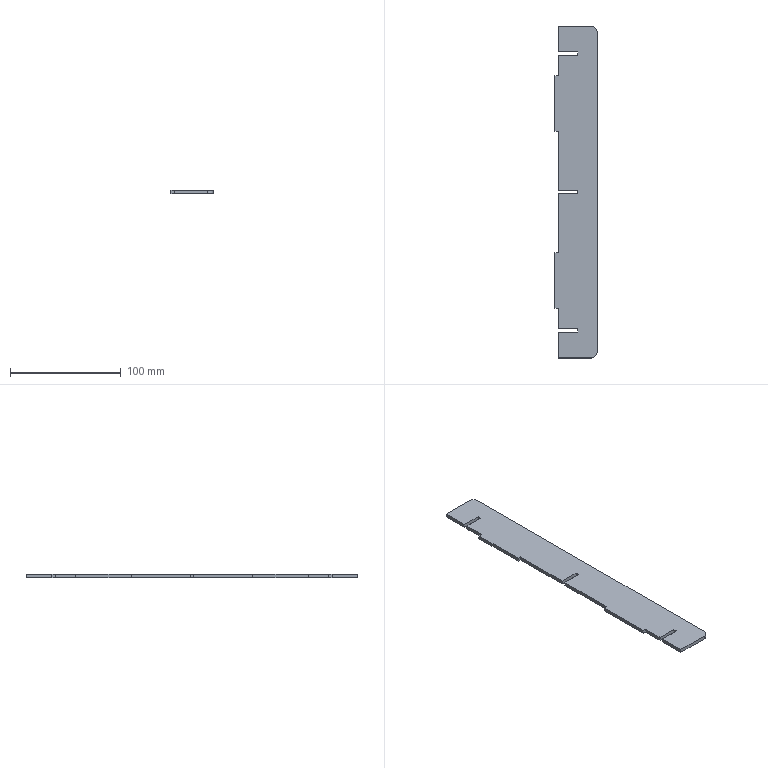Part | SolidWorks | features FlatPattern 1, SMBaseFlange 1, SheetMetal 1 | 1 solid | 28 faces | box 38 x 300 x 3.2 mm | volume 33980 mm3 | plane 26 | cylinder 2 | commonest cylinder face diameters 10 x2
STEP:
#1=CARTESIAN_POINT('',(-214.8,-166.97,0.));
#2=VERTEX_POINT('',#1);
#3=CARTESIAN_POINT('',(-214.8,-190.37,0.));
#4=VERTEX_POINT('',#3);
#5=CARTESIAN_POINT('',(-214.8,-190.37,0.));
#6=DIRECTION('',(0.,-1.,0.));
#7=VECTOR('',#6,1000.);
#8=LINE('',#5,#7);
#9=EDGE_CURVE('',#2,#4,#8,.T.);
#10=ORIENTED_EDGE('',*,*,#9,.F.);
#11=CARTESIAN_POINT('',(-214.8,-166.97,-3.2));
#12=VERTEX_POINT('',#11);
#13=CARTESIAN_POINT('',(-214.8,-166.97,-3.2));
#14=DIRECTION('',(0.,0.,1.));
#15=VECTOR('',#14,1000.);
#16=LINE('',#13,#15);
#17=EDGE_CURVE('',#12,#2,#16,.T.);
#18=ORIENTED_EDGE('',*,*,#17,.F.);
#19=CARTESIAN_POINT('',(-214.8,-190.37,-3.2));
#20=VERTEX_POINT('',#19);
#21=CARTESIAN_POINT('',(-214.8,-190.37,-3.2));
#22=DIRECTION('',(0.,-1.,0.));
#23=VECTOR('',#22,1000.);
#24=LINE('',#21,#23);
#25=EDGE_CURVE('',#12,#20,#24,.T.);
#26=ORIENTED_EDGE('',*,*,#25,.T.);
#27=CARTESIAN_POINT('',(-214.8,-190.37,-3.2));
#28=DIRECTION('',(0.,0.,1.));
#29=VECTOR('',#28,1000.);
#30=LINE('',#27,#29);
#31=EDGE_CURVE('',#20,#4,#30,.T.);
#32=ORIENTED_EDGE('',*,*,#31,.T.);
#33=EDGE_LOOP('',(#10,#18,#26,#32));
#34=FACE_OUTER_BOUND('',#33,.T.);
#35=CARTESIAN_POINT('',(-214.8,-190.37,-3.2));
#36=DIRECTION('',(-1.,0.,0.));
#37=DIRECTION('',(0.,0.,1.));
#38=AXIS2_PLACEMENT_3D('',#35,#36,#37);
#39=PLANE('',#38);
#40=ADVANCED_FACE('',(#34),#39,.T.);
#41=CARTESIAN_POINT('',(-197.05,-166.97,0.));
#42=VERTEX_POINT('',#41);
#43=CARTESIAN_POINT('',(-214.8,-166.97,0.));
#44=DIRECTION('',(-1.,0.,0.));
#45=VECTOR('',#44,1000.);
#46=LINE('',#43,#45);
#47=EDGE_CURVE('',#42,#2,#46,.T.);
#48=ORIENTED_EDGE('',*,*,#47,.F.);
#49=CARTESIAN_POINT('',(-197.05,-166.97,-3.2));
#50=VERTEX_POINT('',#49);
#51=CARTESIAN_POINT('',(-197.05,-166.97,-3.2));
#52=DIRECTION('',(0.,0.,1.));
#53=VECTOR('',#52,1000.);
#54=LINE('',#51,#53);
#55=EDGE_CURVE('',#50,#42,#54,.T.);
#56=ORIENTED_EDGE('',*,*,#55,.F.);
#57=CARTESIAN_POINT('',(-214.8,-166.97,-3.2));
#58=DIRECTION('',(-1.,0.,0.));
#59=VECTOR('',#58,1000.);
#60=LINE('',#57,#59);
#61=EDGE_CURVE('',#50,#12,#60,.T.);
#62=ORIENTED_EDGE('',*,*,#61,.T.);
#63=ORIENTED_EDGE('',*,*,#17,.T.);
#64=EDGE_LOOP('',(#48,#56,#62,#63));
#65=FACE_OUTER_BOUND('',#64,.T.);
#66=CARTESIAN_POINT('',(-214.8,-166.97,-3.2));
#67=DIRECTION('',(0.,1.,0.));
#68=DIRECTION('',(0.,0.,1.));
#69=AXIS2_PLACEMENT_3D('',#66,#67,#68);
#70=PLANE('',#69);
#71=ADVANCED_FACE('',(#65),#70,.T.);
#72=CARTESIAN_POINT('',(-197.05,-163.77,0.));
#73=VERTEX_POINT('',#72);
#74=CARTESIAN_POINT('',(-197.05,-166.97,0.));
#75=DIRECTION('',(0.,-1.,0.));
#76=VECTOR('',#75,1000.);
#77=LINE('',#74,#76);
#78=EDGE_CURVE('',#73,#42,#77,.T.);
#79=ORIENTED_EDGE('',*,*,#78,.F.);
#80=CARTESIAN_POINT('',(-197.05,-163.77,-3.2));
#81=VERTEX_POINT('',#80);
#82=CARTESIAN_POINT('',(-197.05,-163.77,-3.2));
#83=DIRECTION('',(0.,0.,1.));
#84=VECTOR('',#83,1000.);
#85=LINE('',#82,#84);
#86=EDGE_CURVE('',#81,#73,#85,.T.);
#87=ORIENTED_EDGE('',*,*,#86,.F.);
#88=CARTESIAN_POINT('',(-197.05,-166.97,-3.2));
#89=DIRECTION('',(0.,-1.,0.));
#90=VECTOR('',#89,1000.);
#91=LINE('',#88,#90);
#92=EDGE_CURVE('',#81,#50,#91,.T.);
#93=ORIENTED_EDGE('',*,*,#92,.T.);
#94=ORIENTED_EDGE('',*,*,#55,.T.);
#95=EDGE_LOOP('',(#79,#87,#93,#94));
#96=FACE_OUTER_BOUND('',#95,.T.);
#97=CARTESIAN_POINT('',(-197.05,-166.97,-3.2));
#98=DIRECTION('',(-1.,0.,0.));
#99=DIRECTION('',(0.,0.,1.));
#100=AXIS2_PLACEMENT_3D('',#97,#98,#99);
#101=PLANE('',#100);
#102=ADVANCED_FACE('',(#96),#101,.T.);
#103=CARTESIAN_POINT('',(-214.8,-163.77,0.));
#104=VERTEX_POINT('',#103);
#105=CARTESIAN_POINT('',(-197.05,-163.77,0.));
#106=DIRECTION('',(1.,0.,0.));
#107=VECTOR('',#106,1000.);
#108=LINE('',#105,#107);
#109=EDGE_CURVE('',#104,#73,#108,.T.);
#110=ORIENTED_EDGE('',*,*,#109,.F.);
#111=CARTESIAN_POINT('',(-214.8,-163.77,-3.2));
#112=VERTEX_POINT('',#111);
#113=CARTESIAN_POINT('',(-214.8,-163.77,-3.2));
#114=DIRECTION('',(0.,0.,1.));
#115=VECTOR('',#114,1000.);
#116=LINE('',#113,#115);
#117=EDGE_CURVE('',#112,#104,#116,.T.);
#118=ORIENTED_EDGE('',*,*,#117,.F.);
#119=CARTESIAN_POINT('',(-197.05,-163.77,-3.2));
#120=DIRECTION('',(1.,0.,0.));
#121=VECTOR('',#120,1000.);
#122=LINE('',#119,#121);
#123=EDGE_CURVE('',#112,#81,#122,.T.);
#124=ORIENTED_EDGE('',*,*,#123,.T.);
#125=ORIENTED_EDGE('',*,*,#86,.T.);
#126=EDGE_LOOP('',(#110,#118,#124,#125));
#127=FACE_OUTER_BOUND('',#126,.T.);
#128=CARTESIAN_POINT('',(-197.05,-163.77,-3.2));
#129=DIRECTION('',(0.,-1.,0.));
#130=DIRECTION('',(0.,0.,-1.));
#131=AXIS2_PLACEMENT_3D('',#128,#129,#130);
#132=PLANE('',#131);
#133=ADVANCED_FACE('',(#127),#132,.T.);
#134=CARTESIAN_POINT('',(-214.8,-145.37,0.));
#135=VERTEX_POINT('',#134);
#136=CARTESIAN_POINT('',(-214.8,-163.77,0.));
#137=DIRECTION('',(0.,-1.,0.));
#138=VECTOR('',#137,1000.);
#139=LINE('',#136,#138);
#140=EDGE_CURVE('',#135,#104,#139,.T.);
#141=ORIENTED_EDGE('',*,*,#140,.F.);
#142=CARTESIAN_POINT('',(-214.8,-145.37,-3.2));
#143=VERTEX_POINT('',#142);
#144=CARTESIAN_POINT('',(-214.8,-145.37,-3.2));
#145=DIRECTION('',(0.,0.,1.));
#146=VECTOR('',#145,1000.);
#147=LINE('',#144,#146);
#148=EDGE_CURVE('',#143,#135,#147,.T.);
#149=ORIENTED_EDGE('',*,*,#148,.F.);
#150=CARTESIAN_POINT('',(-214.8,-163.77,-3.2));
#151=DIRECTION('',(0.,-1.,0.));
#152=VECTOR('',#151,1000.);
#153=LINE('',#150,#152);
#154=EDGE_CURVE('',#143,#112,#153,.T.);
#155=ORIENTED_EDGE('',*,*,#154,.T.);
#156=ORIENTED_EDGE('',*,*,#117,.T.);
#157=EDGE_LOOP('',(#141,#149,#155,#156));
#158=FACE_OUTER_BOUND('',#157,.T.);
#159=CARTESIAN_POINT('',(-214.8,-163.77,-3.2));
#160=DIRECTION('',(-1.,0.,0.));
#161=DIRECTION('',(0.,0.,1.));
#162=AXIS2_PLACEMENT_3D('',#159,#160,#161);
#163=PLANE('',#162);
#164=ADVANCED_FACE('',(#158),#163,.T.);
#165=CARTESIAN_POINT('',(-217.8,-145.37,0.));
#166=VERTEX_POINT('',#165);
#167=CARTESIAN_POINT('',(-214.8,-145.37,0.));
#168=DIRECTION('',(1.,0.,0.));
#169=VECTOR('',#168,1000.);
#170=LINE('',#167,#169);
#171=EDGE_CURVE('',#166,#135,#170,.T.);
#172=ORIENTED_EDGE('',*,*,#171,.F.);
#173=CARTESIAN_POINT('',(-217.8,-145.37,-3.2));
#174=VERTEX_POINT('',#173);
#175=CARTESIAN_POINT('',(-217.8,-145.37,-3.2));
#176=DIRECTION('',(0.,0.,1.));
#177=VECTOR('',#176,1000.);
#178=LINE('',#175,#177);
#179=EDGE_CURVE('',#174,#166,#178,.T.);
#180=ORIENTED_EDGE('',*,*,#179,.F.);
#181=CARTESIAN_POINT('',(-214.8,-145.37,-3.2));
#182=DIRECTION('',(1.,0.,0.));
#183=VECTOR('',#182,1000.);
#184=LINE('',#181,#183);
#185=EDGE_CURVE('',#174,#143,#184,.T.);
#186=ORIENTED_EDGE('',*,*,#185,.T.);
#187=ORIENTED_EDGE('',*,*,#148,.T.);
#188=EDGE_LOOP('',(#172,#180,#186,#187));
#189=FACE_OUTER_BOUND('',#188,.T.);
#190=CARTESIAN_POINT('',(-214.8,-145.37,-3.2));
#191=DIRECTION('',(0.,-1.,0.));
#192=DIRECTION('',(0.,0.,-1.));
#193=AXIS2_PLACEMENT_3D('',#190,#191,#192);
#194=PLANE('',#193);
#195=ADVANCED_FACE('',(#189),#194,.T.);
#196=CARTESIAN_POINT('',(-217.8,-95.37,0.));
#197=VERTEX_POINT('',#196);
#198=CARTESIAN_POINT('',(-217.8,-145.37,0.));
#199=DIRECTION('',(0.,-1.,0.));
#200=VECTOR('',#199,1000.);
#201=LINE('',#198,#200);
#202=EDGE_CURVE('',#197,#166,#201,.T.);
#203=ORIENTED_EDGE('',*,*,#202,.F.);
#204=CARTESIAN_POINT('',(-217.8,-95.37,-3.2));
#205=VERTEX_POINT('',#204);
#206=CARTESIAN_POINT('',(-217.8,-95.37,-3.2));
#207=DIRECTION('',(0.,0.,1.));
#208=VECTOR('',#207,1000.);
#209=LINE('',#206,#208);
#210=EDGE_CURVE('',#205,#197,#209,.T.);
#211=ORIENTED_EDGE('',*,*,#210,.F.);
#212=CARTESIAN_POINT('',(-217.8,-145.37,-3.2));
#213=DIRECTION('',(0.,-1.,0.));
#214=VECTOR('',#213,1000.);
#215=LINE('',#212,#214);
#216=EDGE_CURVE('',#205,#174,#215,.T.);
#217=ORIENTED_EDGE('',*,*,#216,.T.);
#218=ORIENTED_EDGE('',*,*,#179,.T.);
#219=EDGE_LOOP('',(#203,#211,#217,#218));
#220=FACE_OUTER_BOUND('',#219,.T.);
#221=CARTESIAN_POINT('',(-217.8,-145.37,-3.2));
#222=DIRECTION('',(-1.,0.,0.));
#223=DIRECTION('',(0.,0.,1.));
#224=AXIS2_PLACEMENT_3D('',#221,#222,#223);
#225=PLANE('',#224);
#226=ADVANCED_FACE('',(#220),#225,.T.);
#227=CARTESIAN_POINT('',(-214.8,-95.37,0.));
#228=VERTEX_POINT('',#227);
#229=CARTESIAN_POINT('',(-217.8,-95.37,0.));
#230=DIRECTION('',(-1.,0.,0.));
#231=VECTOR('',#230,1000.);
#232=LINE('',#229,#231);
#233=EDGE_CURVE('',#228,#197,#232,.T.);
#234=ORIENTED_EDGE('',*,*,#233,.F.);
#235=CARTESIAN_POINT('',(-214.8,-95.37,-3.2));
#236=VERTEX_POINT('',#235);
#237=CARTESIAN_POINT('',(-214.8,-95.37,-3.2));
#238=DIRECTION('',(0.,0.,1.));
#239=VECTOR('',#238,1000.);
#240=LINE('',#237,#239);
#241=EDGE_CURVE('',#236,#228,#240,.T.);
#242=ORIENTED_EDGE('',*,*,#241,.F.);
#243=CARTESIAN_POINT('',(-217.8,-95.37,-3.2));
#244=DIRECTION('',(-1.,0.,0.));
#245=VECTOR('',#244,1000.);
#246=LINE('',#243,#245);
#247=EDGE_CURVE('',#236,#205,#246,.T.);
#248=ORIENTED_EDGE('',*,*,#247,.T.);
#249=ORIENTED_EDGE('',*,*,#210,.T.);
#250=EDGE_LOOP('',(#234,#242,#248,#249));
#251=FACE_OUTER_BOUND('',#250,.T.);
#252=CARTESIAN_POINT('',(-217.8,-95.37,-3.2));
#253=DIRECTION('',(0.,1.,0.));
#254=DIRECTION('',(0.,0.,1.));
#255=AXIS2_PLACEMENT_3D('',#252,#253,#254);
#256=PLANE('',#255);
#257=ADVANCED_FACE('',(#251),#256,.T.);
#258=CARTESIAN_POINT('',(-214.8,-41.97,0.));
#259=VERTEX_POINT('',#258);
#260=CARTESIAN_POINT('',(-214.8,-95.37,0.));
#261=DIRECTION('',(0.,-1.,0.));
#262=VECTOR('',#261,1000.);
#263=LINE('',#260,#262);
#264=EDGE_CURVE('',#259,#228,#263,.T.);
#265=ORIENTED_EDGE('',*,*,#264,.F.);
#266=CARTESIAN_POINT('',(-214.8,-41.97,-3.2));
#267=VERTEX_POINT('',#266);
#268=CARTESIAN_POINT('',(-214.8,-41.97,-3.2));
#269=DIRECTION('',(0.,0.,1.));
#270=VECTOR('',#269,1000.);
#271=LINE('',#268,#270);
#272=EDGE_CURVE('',#267,#259,#271,.T.);
#273=ORIENTED_EDGE('',*,*,#272,.F.);
#274=CARTESIAN_POINT('',(-214.8,-95.37,-3.2));
#275=DIRECTION('',(0.,-1.,0.));
#276=VECTOR('',#275,1000.);
#277=LINE('',#274,#276);
#278=EDGE_CURVE('',#267,#236,#277,.T.);
#279=ORIENTED_EDGE('',*,*,#278,.T.);
#280=ORIENTED_EDGE('',*,*,#241,.T.);
#281=EDGE_LOOP('',(#265,#273,#279,#280));
#282=FACE_OUTER_BOUND('',#281,.T.);
#283=CARTESIAN_POINT('',(-214.8,-95.37,-3.2));
#284=DIRECTION('',(-1.,0.,0.));
#285=DIRECTION('',(0.,0.,1.));
#286=AXIS2_PLACEMENT_3D('',#283,#284,#285);
#287=PLANE('',#286);
#288=ADVANCED_FACE('',(#282),#287,.T.);
#289=CARTESIAN_POINT('',(-197.05,-41.97,0.));
#290=VERTEX_POINT('',#289);
#291=CARTESIAN_POINT('',(-214.8,-41.97,0.));
#292=DIRECTION('',(-1.,0.,0.));
#293=VECTOR('',#292,1000.);
#294=LINE('',#291,#293);
#295=EDGE_CURVE('',#290,#259,#294,.T.);
#296=ORIENTED_EDGE('',*,*,#295,.F.);
#297=CARTESIAN_POINT('',(-197.05,-41.97,-3.2));
#298=VERTEX_POINT('',#297);
#299=CARTESIAN_POINT('',(-197.05,-41.97,-3.2));
#300=DIRECTION('',(0.,0.,1.));
#301=VECTOR('',#300,1000.);
#302=LINE('',#299,#301);
#303=EDGE_CURVE('',#298,#290,#302,.T.);
#304=ORIENTED_EDGE('',*,*,#303,.F.);
#305=CARTESIAN_POINT('',(-214.8,-41.97,-3.2));
#306=DIRECTION('',(-1.,0.,0.));
#307=VECTOR('',#306,1000.);
#308=LINE('',#305,#307);
#309=EDGE_CURVE('',#298,#267,#308,.T.);
#310=ORIENTED_EDGE('',*,*,#309,.T.);
#311=ORIENTED_EDGE('',*,*,#272,.T.);
#312=EDGE_LOOP('',(#296,#304,#310,#311));
#313=FACE_OUTER_BOUND('',#312,.T.);
#314=CARTESIAN_POINT('',(-214.8,-41.97,-3.2));
#315=DIRECTION('',(0.,1.,0.));
#316=DIRECTION('',(0.,0.,1.));
#317=AXIS2_PLACEMENT_3D('',#314,#315,#316);
#318=PLANE('',#317);
#319=ADVANCED_FACE('',(#313),#318,.T.);
#320=CARTESIAN_POINT('',(-197.05,-38.77,0.));
#321=VERTEX_POINT('',#320);
#322=CARTESIAN_POINT('',(-197.05,-41.97,0.));
#323=DIRECTION('',(0.,-1.,0.));
#324=VECTOR('',#323,1000.);
#325=LINE('',#322,#324);
#326=EDGE_CURVE('',#321,#290,#325,.T.);
#327=ORIENTED_EDGE('',*,*,#326,.F.);
#328=CARTESIAN_POINT('',(-197.05,-38.77,-3.2));
#329=VERTEX_POINT('',#328);
#330=CARTESIAN_POINT('',(-197.05,-38.77,-3.2));
#331=DIRECTION('',(0.,0.,1.));
#332=VECTOR('',#331,1000.);
#333=LINE('',#330,#332);
#334=EDGE_CURVE('',#329,#321,#333,.T.);
#335=ORIENTED_EDGE('',*,*,#334,.F.);
#336=CARTESIAN_POINT('',(-197.05,-41.97,-3.2));
#337=DIRECTION('',(0.,-1.,0.));
#338=VECTOR('',#337,1000.);
#339=LINE('',#336,#338);
#340=EDGE_CURVE('',#329,#298,#339,.T.);
#341=ORIENTED_EDGE('',*,*,#340,.T.);
#342=ORIENTED_EDGE('',*,*,#303,.T.);
#343=EDGE_LOOP('',(#327,#335,#341,#342));
#344=FACE_OUTER_BOUND('',#343,.T.);
#345=CARTESIAN_POINT('',(-197.05,-41.97,-3.2));
#346=DIRECTION('',(-1.,0.,0.));
#347=DIRECTION('',(0.,0.,1.));
#348=AXIS2_PLACEMENT_3D('',#345,#346,#347);
#349=PLANE('',#348);
#350=ADVANCED_FACE('',(#344),#349,.T.);
#351=CARTESIAN_POINT('',(-214.8,-38.77,0.));
#352=VERTEX_POINT('',#351);
#353=CARTESIAN_POINT('',(-197.05,-38.77,0.));
#354=DIRECTION('',(1.,0.,0.));
#355=VECTOR('',#354,1000.);
#356=LINE('',#353,#355);
#357=EDGE_CURVE('',#352,#321,#356,.T.);
#358=ORIENTED_EDGE('',*,*,#357,.F.);
#359=CARTESIAN_POINT('',(-214.8,-38.77,-3.2));
#360=VERTEX_POINT('',#359);
#361=CARTESIAN_POINT('',(-214.8,-38.77,-3.2));
#362=DIRECTION('',(0.,0.,1.));
#363=VECTOR('',#362,1000.);
#364=LINE('',#361,#363);
#365=EDGE_CURVE('',#360,#352,#364,.T.);
#366=ORIENTED_EDGE('',*,*,#365,.F.);
#367=CARTESIAN_POINT('',(-197.05,-38.77,-3.2));
#368=DIRECTION('',(1.,0.,0.));
#369=VECTOR('',#368,1000.);
#370=LINE('',#367,#369);
#371=EDGE_CURVE('',#360,#329,#370,.T.);
#372=ORIENTED_EDGE('',*,*,#371,.T.);
#373=ORIENTED_EDGE('',*,*,#334,.T.);
#374=EDGE_LOOP('',(#358,#366,#372,#373));
#375=FACE_OUTER_BOUND('',#374,.T.);
#376=CARTESIAN_POINT('',(-197.05,-38.77,-3.2));
#377=DIRECTION('',(0.,-1.,0.));
#378=DIRECTION('',(0.,0.,-1.));
#379=AXIS2_PLACEMENT_3D('',#376,#377,#378);
#380=PLANE('',#379);
#381=ADVANCED_FACE('',(#375),#380,.T.);
#382=CARTESIAN_POINT('',(-214.8,14.63,0.));
#383=VERTEX_POINT('',#382);
#384=CARTESIAN_POINT('',(-214.8,-38.77,0.));
#385=DIRECTION('',(0.,-1.,0.));
#386=VECTOR('',#385,1000.);
#387=LINE('',#384,#386);
#388=EDGE_CURVE('',#383,#352,#387,.T.);
#389=ORIENTED_EDGE('',*,*,#388,.F.);
#390=CARTESIAN_POINT('',(-214.8,14.63,-3.2));
#391=VERTEX_POINT('',#390);
#392=CARTESIAN_POINT('',(-214.8,14.63,-3.2));
#393=DIRECTION('',(0.,0.,1.));
#394=VECTOR('',#393,1000.);
#395=LINE('',#392,#394);
#396=EDGE_CURVE('',#391,#383,#395,.T.);
#397=ORIENTED_EDGE('',*,*,#396,.F.);
#398=CARTESIAN_POINT('',(-214.8,-38.77,-3.2));
#399=DIRECTION('',(0.,-1.,0.));
#400=VECTOR('',#399,1000.);
#401=LINE('',#398,#400);
#402=EDGE_CURVE('',#391,#360,#401,.T.);
#403=ORIENTED_EDGE('',*,*,#402,.T.);
#404=ORIENTED_EDGE('',*,*,#365,.T.);
#405=EDGE_LOOP('',(#389,#397,#403,#404));
#406=FACE_OUTER_BOUND('',#405,.T.);
#407=CARTESIAN_POINT('',(-214.8,-38.77,-3.2));
#408=DIRECTION('',(-1.,0.,0.));
#409=DIRECTION('',(0.,0.,1.));
#410=AXIS2_PLACEMENT_3D('',#407,#408,#409);
#411=PLANE('',#410);
#412=ADVANCED_FACE('',(#406),#411,.T.);
#413=CARTESIAN_POINT('',(-217.8,14.63,0.));
#414=VERTEX_POINT('',#413);
#415=CARTESIAN_POINT('',(-217.8,14.63,0.));
#416=DIRECTION('',(1.,0.,0.));
#417=VECTOR('',#416,1000.);
#418=LINE('',#415,#417);
#419=EDGE_CURVE('',#414,#383,#418,.T.);
#420=ORIENTED_EDGE('',*,*,#419,.F.);
#421=CARTESIAN_POINT('',(-217.8,14.63,-3.2));
#422=VERTEX_POINT('',#421);
#423=CARTESIAN_POINT('',(-217.8,14.63,-3.2));
#424=DIRECTION('',(0.,0.,1.));
#425=VECTOR('',#424,1000.);
#426=LINE('',#423,#425);
#427=EDGE_CURVE('',#422,#414,#426,.T.);
#428=ORIENTED_EDGE('',*,*,#427,.F.);
#429=CARTESIAN_POINT('',(-217.8,14.63,-3.2));
#430=DIRECTION('',(1.,0.,0.));
#431=VECTOR('',#430,1000.);
#432=LINE('',#429,#431);
#433=EDGE_CURVE('',#422,#391,#432,.T.);
#434=ORIENTED_EDGE('',*,*,#433,.T.);
#435=ORIENTED_EDGE('',*,*,#396,.T.);
#436=EDGE_LOOP('',(#420,#428,#434,#435));
#437=FACE_OUTER_BOUND('',#436,.T.);
#438=CARTESIAN_POINT('',(-217.8,14.63,-3.2));
#439=DIRECTION('',(0.,-1.,0.));
#440=DIRECTION('',(1.,0.,0.));
#441=AXIS2_PLACEMENT_3D('',#438,#439,#440);
#442=PLANE('',#441);
#443=ADVANCED_FACE('',(#437),#442,.T.);
#444=CARTESIAN_POINT('',(-217.8,64.63,0.));
#445=VERTEX_POINT('',#444);
#446=CARTESIAN_POINT('',(-217.8,64.63,0.));
#447=DIRECTION('',(0.,-1.,0.));
#448=VECTOR('',#447,1000.);
#449=LINE('',#446,#448);
#450=EDGE_CURVE('',#445,#414,#449,.T.);
#451=ORIENTED_EDGE('',*,*,#450,.F.);
#452=CARTESIAN_POINT('',(-217.8,64.63,-3.2));
#453=VERTEX_POINT('',#452);
#454=CARTESIAN_POINT('',(-217.8,64.63,-3.2));
#455=DIRECTION('',(0.,0.,1.));
#456=VECTOR('',#455,1000.);
#457=LINE('',#454,#456);
#458=EDGE_CURVE('',#453,#445,#457,.T.);
#459=ORIENTED_EDGE('',*,*,#458,.F.);
#460=CARTESIAN_POINT('',(-217.8,64.63,-3.2));
#461=DIRECTION('',(0.,-1.,0.));
#462=VECTOR('',#461,1000.);
#463=LINE('',#460,#462);
#464=EDGE_CURVE('',#453,#422,#463,.T.);
#465=ORIENTED_EDGE('',*,*,#464,.T.);
#466=ORIENTED_EDGE('',*,*,#427,.T.);
#467=EDGE_LOOP('',(#451,#459,#465,#466));
#468=FACE_OUTER_BOUND('',#467,.T.);
#469=CARTESIAN_POINT('',(-217.8,64.63,-3.2));
#470=DIRECTION('',(-1.,0.,0.));
#471=DIRECTION('',(0.,-1.,0.));
#472=AXIS2_PLACEMENT_3D('',#469,#470,#471);
#473=PLANE('',#472);
#474=ADVANCED_FACE('',(#468),#473,.T.);
#475=CARTESIAN_POINT('',(-214.8,64.63,0.));
#476=VERTEX_POINT('',#475);
#477=CARTESIAN_POINT('',(-214.8,64.63,0.));
#478=DIRECTION('',(-1.,0.,0.));
#479=VECTOR('',#478,1000.);
#480=LINE('',#477,#479);
#481=EDGE_CURVE('',#476,#445,#480,.T.);
#482=ORIENTED_EDGE('',*,*,#481,.F.);
#483=CARTESIAN_POINT('',(-214.8,64.63,-3.2));
#484=VERTEX_POINT('',#483);
#485=CARTESIAN_POINT('',(-214.8,64.63,-3.2));
#486=DIRECTION('',(0.,0.,1.));
#487=VECTOR('',#486,1000.);
#488=LINE('',#485,#487);
#489=EDGE_CURVE('',#484,#476,#488,.T.);
#490=ORIENTED_EDGE('',*,*,#489,.F.);
#491=CARTESIAN_POINT('',(-214.8,64.63,-3.2));
#492=DIRECTION('',(-1.,0.,0.));
#493=VECTOR('',#492,1000.);
#494=LINE('',#491,#493);
#495=EDGE_CURVE('',#484,#453,#494,.T.);
#496=ORIENTED_EDGE('',*,*,#495,.T.);
#497=ORIENTED_EDGE('',*,*,#458,.T.);
#498=EDGE_LOOP('',(#482,#490,#496,#497));
#499=FACE_OUTER_BOUND('',#498,.T.);
#500=CARTESIAN_POINT('',(-214.8,64.63,-3.2));
#501=DIRECTION('',(0.,1.,0.));
#502=DIRECTION('',(0.,0.,1.));
#503=AXIS2_PLACEMENT_3D('',#500,#501,#502);
#504=PLANE('',#503);
#505=ADVANCED_FACE('',(#499),#504,.T.);
#506=CARTESIAN_POINT('',(-214.8,83.03,0.));
#507=VERTEX_POINT('',#506);
#508=CARTESIAN_POINT('',(-214.8,64.63,0.));
#509=DIRECTION('',(0.,-1.,0.));
#510=VECTOR('',#509,1000.);
#511=LINE('',#508,#510);
#512=EDGE_CURVE('',#507,#476,#511,.T.);
#513=ORIENTED_EDGE('',*,*,#512,.F.);
#514=CARTESIAN_POINT('',(-214.8,83.03,-3.2));
#515=VERTEX_POINT('',#514);
#516=CARTESIAN_POINT('',(-214.8,83.03,-3.2));
#517=DIRECTION('',(0.,0.,1.));
#518=VECTOR('',#517,1000.);
#519=LINE('',#516,#518);
#520=EDGE_CURVE('',#515,#507,#519,.T.);
#521=ORIENTED_EDGE('',*,*,#520,.F.);
#522=CARTESIAN_POINT('',(-214.8,64.63,-3.2));
#523=DIRECTION('',(0.,-1.,0.));
#524=VECTOR('',#523,1000.);
#525=LINE('',#522,#524);
#526=EDGE_CURVE('',#515,#484,#525,.T.);
#527=ORIENTED_EDGE('',*,*,#526,.T.);
#528=ORIENTED_EDGE('',*,*,#489,.T.);
#529=EDGE_LOOP('',(#513,#521,#527,#528));
#530=FACE_OUTER_BOUND('',#529,.T.);
#531=CARTESIAN_POINT('',(-214.8,64.63,-3.2));
#532=DIRECTION('',(-1.,0.,0.));
#533=DIRECTION('',(0.,0.,1.));
#534=AXIS2_PLACEMENT_3D('',#531,#532,#533);
#535=PLANE('',#534);
#536=ADVANCED_FACE('',(#530),#535,.T.);
#537=CARTESIAN_POINT('',(-197.05,83.03,0.));
#538=VERTEX_POINT('',#537);
#539=CARTESIAN_POINT('',(-214.8,83.03,0.));
#540=DIRECTION('',(-1.,0.,0.));
#541=VECTOR('',#540,1000.);
#542=LINE('',#539,#541);
#543=EDGE_CURVE('',#538,#507,#542,.T.);
#544=ORIENTED_EDGE('',*,*,#543,.F.);
#545=CARTESIAN_POINT('',(-197.05,83.03,-3.2));
#546=VERTEX_POINT('',#545);
#547=CARTESIAN_POINT('',(-197.05,83.03,-3.2));
#548=DIRECTION('',(0.,0.,1.));
#549=VECTOR('',#548,1000.);
#550=LINE('',#547,#549);
#551=EDGE_CURVE('',#546,#538,#550,.T.);
#552=ORIENTED_EDGE('',*,*,#551,.F.);
#553=CARTESIAN_POINT('',(-214.8,83.03,-3.2));
#554=DIRECTION('',(-1.,0.,0.));
#555=VECTOR('',#554,1000.);
#556=LINE('',#553,#555);
#557=EDGE_CURVE('',#546,#515,#556,.T.);
#558=ORIENTED_EDGE('',*,*,#557,.T.);
#559=ORIENTED_EDGE('',*,*,#520,.T.);
#560=EDGE_LOOP('',(#544,#552,#558,#559));
#561=FACE_OUTER_BOUND('',#560,.T.);
#562=CARTESIAN_POINT('',(-214.8,83.03,-3.2));
#563=DIRECTION('',(0.,1.,0.));
#564=DIRECTION('',(0.,0.,1.));
#565=AXIS2_PLACEMENT_3D('',#562,#563,#564);
#566=PLANE('',#565);
#567=ADVANCED_FACE('',(#561),#566,.T.);
#568=CARTESIAN_POINT('',(-197.05,86.23,0.));
#569=VERTEX_POINT('',#568);
#570=CARTESIAN_POINT('',(-197.05,83.03,0.));
#571=DIRECTION('',(0.,-1.,0.));
#572=VECTOR('',#571,1000.);
#573=LINE('',#570,#572);
#574=EDGE_CURVE('',#569,#538,#573,.T.);
#575=ORIENTED_EDGE('',*,*,#574,.F.);
#576=CARTESIAN_POINT('',(-197.05,86.23,-3.2));
#577=VERTEX_POINT('',#576);
#578=CARTESIAN_POINT('',(-197.05,86.23,-3.2));
#579=DIRECTION('',(0.,0.,1.));
#580=VECTOR('',#579,1000.);
#581=LINE('',#578,#580);
#582=EDGE_CURVE('',#577,#569,#581,.T.);
#583=ORIENTED_EDGE('',*,*,#582,.F.);
#584=CARTESIAN_POINT('',(-197.05,83.03,-3.2));
#585=DIRECTION('',(0.,-1.,0.));
#586=VECTOR('',#585,1000.);
#587=LINE('',#584,#586);
#588=EDGE_CURVE('',#577,#546,#587,.T.);
#589=ORIENTED_EDGE('',*,*,#588,.T.);
#590=ORIENTED_EDGE('',*,*,#551,.T.);
#591=EDGE_LOOP('',(#575,#583,#589,#590));
#592=FACE_OUTER_BOUND('',#591,.T.);
#593=CARTESIAN_POINT('',(-197.05,83.03,-3.2));
#594=DIRECTION('',(-1.,0.,0.));
#595=DIRECTION('',(0.,0.,1.));
#596=AXIS2_PLACEMENT_3D('',#593,#594,#595);
#597=PLANE('',#596);
#598=ADVANCED_FACE('',(#592),#597,.T.);
#599=CARTESIAN_POINT('',(-214.8,86.23,0.));
#600=VERTEX_POINT('',#599);
#601=CARTESIAN_POINT('',(-197.05,86.23,0.));
#602=DIRECTION('',(1.,0.,0.));
#603=VECTOR('',#602,1000.);
#604=LINE('',#601,#603);
#605=EDGE_CURVE('',#600,#569,#604,.T.);
#606=ORIENTED_EDGE('',*,*,#605,.F.);
#607=CARTESIAN_POINT('',(-214.8,86.23,-3.2));
#608=VERTEX_POINT('',#607);
#609=CARTESIAN_POINT('',(-214.8,86.23,-3.2));
#610=DIRECTION('',(0.,0.,1.));
#611=VECTOR('',#610,1000.);
#612=LINE('',#609,#611);
#613=EDGE_CURVE('',#608,#600,#612,.T.);
#614=ORIENTED_EDGE('',*,*,#613,.F.);
#615=CARTESIAN_POINT('',(-197.05,86.23,-3.2));
#616=DIRECTION('',(1.,0.,0.));
#617=VECTOR('',#616,1000.);
#618=LINE('',#615,#617);
#619=EDGE_CURVE('',#608,#577,#618,.T.);
#620=ORIENTED_EDGE('',*,*,#619,.T.);
#621=ORIENTED_EDGE('',*,*,#582,.T.);
#622=EDGE_LOOP('',(#606,#614,#620,#621));
#623=FACE_OUTER_BOUND('',#622,.T.);
#624=CARTESIAN_POINT('',(-197.05,86.23,-3.2));
#625=DIRECTION('',(0.,-1.,0.));
#626=DIRECTION('',(0.,0.,-1.));
#627=AXIS2_PLACEMENT_3D('',#624,#625,#626);
#628=PLANE('',#627);
#629=ADVANCED_FACE('',(#623),#628,.T.);
#630=CARTESIAN_POINT('',(-214.8,109.63,0.));
#631=VERTEX_POINT('',#630);
#632=CARTESIAN_POINT('',(-214.8,86.23,0.));
#633=DIRECTION('',(0.,-1.,0.));
#634=VECTOR('',#633,1000.);
#635=LINE('',#632,#634);
#636=EDGE_CURVE('',#631,#600,#635,.T.);
#637=ORIENTED_EDGE('',*,*,#636,.F.);
#638=CARTESIAN_POINT('',(-214.8,109.63,-3.2));
#639=VERTEX_POINT('',#638);
#640=CARTESIAN_POINT('',(-214.8,109.63,-3.2));
#641=DIRECTION('',(0.,0.,1.));
#642=VECTOR('',#641,1000.);
#643=LINE('',#640,#642);
#644=EDGE_CURVE('',#639,#631,#643,.T.);
#645=ORIENTED_EDGE('',*,*,#644,.F.);
#646=CARTESIAN_POINT('',(-214.8,86.23,-3.2));
#647=DIRECTION('',(0.,-1.,0.));
#648=VECTOR('',#647,1000.);
#649=LINE('',#646,#648);
#650=EDGE_CURVE('',#639,#608,#649,.T.);
#651=ORIENTED_EDGE('',*,*,#650,.T.);
#652=ORIENTED_EDGE('',*,*,#613,.T.);
#653=EDGE_LOOP('',(#637,#645,#651,#652));
#654=FACE_OUTER_BOUND('',#653,.T.);
#655=CARTESIAN_POINT('',(-214.8,86.23,-3.2));
#656=DIRECTION('',(-1.,0.,0.));
#657=DIRECTION('',(0.,0.,1.));
#658=AXIS2_PLACEMENT_3D('',#655,#656,#657);
#659=PLANE('',#658);
#660=ADVANCED_FACE('',(#654),#659,.T.);
#661=CARTESIAN_POINT('',(-184.8,109.63,0.));
#662=VERTEX_POINT('',#661);
#663=CARTESIAN_POINT('',(-214.8,109.63,0.));
#664=DIRECTION('',(-1.,0.,0.));
#665=VECTOR('',#664,1000.);
#666=LINE('',#663,#665);
#667=EDGE_CURVE('',#662,#631,#666,.T.);
#668=ORIENTED_EDGE('',*,*,#667,.F.);
#669=CARTESIAN_POINT('',(-184.8,109.63,-3.2));
#670=VERTEX_POINT('',#669);
#671=CARTESIAN_POINT('',(-184.8,109.63,-3.2));
#672=DIRECTION('',(0.,0.,1.));
#673=VECTOR('',#672,1000.);
#674=LINE('',#671,#673);
#675=EDGE_CURVE('',#670,#662,#674,.T.);
#676=ORIENTED_EDGE('',*,*,#675,.F.);
#677=CARTESIAN_POINT('',(-214.8,109.63,-3.2));
#678=DIRECTION('',(-1.,0.,0.));
#679=VECTOR('',#678,1000.);
#680=LINE('',#677,#679);
#681=EDGE_CURVE('',#670,#639,#680,.T.);
#682=ORIENTED_EDGE('',*,*,#681,.T.);
#683=ORIENTED_EDGE('',*,*,#644,.T.);
#684=EDGE_LOOP('',(#668,#676,#682,#683));
#685=FACE_OUTER_BOUND('',#684,.T.);
#686=CARTESIAN_POINT('',(-214.8,109.63,-3.2));
#687=DIRECTION('',(0.,1.,0.));
#688=DIRECTION('',(0.,0.,1.));
#689=AXIS2_PLACEMENT_3D('',#686,#687,#688);
#690=PLANE('',#689);
#691=ADVANCED_FACE('',(#685),#690,.T.);
#692=CARTESIAN_POINT('',(-179.8,104.63,0.));
#693=VERTEX_POINT('',#692);
#694=CARTESIAN_POINT('',(-184.8,104.63,0.));
#695=DIRECTION('',(0.,0.,1.));
#696=DIRECTION('',(-1.,0.,0.));
#697=AXIS2_PLACEMENT_3D('',#694,#695,#696);
#698=CIRCLE('',#697,5.);
#699=EDGE_CURVE('',#693,#662,#698,.T.);
#700=ORIENTED_EDGE('',*,*,#699,.F.);
#701=CARTESIAN_POINT('',(-179.8,104.63,-3.2));
#702=VERTEX_POINT('',#701);
#703=CARTESIAN_POINT('',(-179.8,104.63,-3.2));
#704=DIRECTION('',(0.,0.,1.));
#705=VECTOR('',#704,1000.);
#706=LINE('',#703,#705);
#707=EDGE_CURVE('',#702,#693,#706,.T.);
#708=ORIENTED_EDGE('',*,*,#707,.F.);
#709=CARTESIAN_POINT('',(-184.8,104.63,-3.2));
#710=DIRECTION('',(0.,0.,1.));
#711=DIRECTION('',(-1.,0.,0.));
#712=AXIS2_PLACEMENT_3D('',#709,#710,#711);
#713=CIRCLE('',#712,5.);
#714=EDGE_CURVE('',#702,#670,#713,.T.);
#715=ORIENTED_EDGE('',*,*,#714,.T.);
#716=ORIENTED_EDGE('',*,*,#675,.T.);
#717=EDGE_LOOP('',(#700,#708,#715,#716));
#718=FACE_OUTER_BOUND('',#717,.T.);
#719=CARTESIAN_POINT('',(-184.8,104.63,-3.2));
#720=DIRECTION('',(0.,0.,1.));
#721=DIRECTION('',(1.,0.,0.));
#722=AXIS2_PLACEMENT_3D('',#719,#720,#721);
#723=CYLINDRICAL_SURFACE('',#722,5.);
#724=ADVANCED_FACE('',(#718),#723,.T.);
#725=CARTESIAN_POINT('',(-179.8,-185.37,0.));
#726=VERTEX_POINT('',#725);
#727=CARTESIAN_POINT('',(-179.8,-185.37,0.));
#728=DIRECTION('',(0.,1.,0.));
#729=VECTOR('',#728,1000.);
#730=LINE('',#727,#729);
#731=EDGE_CURVE('',#726,#693,#730,.T.);
#732=ORIENTED_EDGE('',*,*,#731,.F.);
#733=CARTESIAN_POINT('',(-179.8,-185.37,-3.2));
#734=VERTEX_POINT('',#733);
#735=CARTESIAN_POINT('',(-179.8,-185.37,-3.2));
#736=DIRECTION('',(0.,0.,1.));
#737=VECTOR('',#736,1000.);
#738=LINE('',#735,#737);
#739=EDGE_CURVE('',#734,#726,#738,.T.);
#740=ORIENTED_EDGE('',*,*,#739,.F.);
#741=CARTESIAN_POINT('',(-179.8,-185.37,-3.2));
#742=DIRECTION('',(0.,1.,0.));
#743=VECTOR('',#742,1000.);
#744=LINE('',#741,#743);
#745=EDGE_CURVE('',#734,#702,#744,.T.);
#746=ORIENTED_EDGE('',*,*,#745,.T.);
#747=ORIENTED_EDGE('',*,*,#707,.T.);
#748=EDGE_LOOP('',(#732,#740,#746,#747));
#749=FACE_OUTER_BOUND('',#748,.T.);
#750=CARTESIAN_POINT('',(-179.8,-185.37,-3.2));
#751=DIRECTION('',(1.,0.,0.));
#752=DIRECTION('',(0.,0.,-1.));
#753=AXIS2_PLACEMENT_3D('',#750,#751,#752);
#754=PLANE('',#753);
#755=ADVANCED_FACE('',(#749),#754,.T.);
#756=CARTESIAN_POINT('',(-184.8,-190.37,0.));
#757=VERTEX_POINT('',#756);
#758=CARTESIAN_POINT('',(-184.8,-185.37,0.));
#759=DIRECTION('',(0.,0.,1.));
#760=DIRECTION('',(1.,0.,0.));
#761=AXIS2_PLACEMENT_3D('',#758,#759,#760);
#762=CIRCLE('',#761,5.);
#763=EDGE_CURVE('',#757,#726,#762,.T.);
#764=ORIENTED_EDGE('',*,*,#763,.F.);
#765=CARTESIAN_POINT('',(-184.8,-190.37,-3.2));
#766=VERTEX_POINT('',#765);
#767=CARTESIAN_POINT('',(-184.8,-190.37,-3.2));
#768=DIRECTION('',(0.,0.,1.));
#769=VECTOR('',#768,1000.);
#770=LINE('',#767,#769);
#771=EDGE_CURVE('',#766,#757,#770,.T.);
#772=ORIENTED_EDGE('',*,*,#771,.F.);
#773=CARTESIAN_POINT('',(-184.8,-185.37,-3.2));
#774=DIRECTION('',(0.,0.,1.));
#775=DIRECTION('',(1.,0.,0.));
#776=AXIS2_PLACEMENT_3D('',#773,#774,#775);
#777=CIRCLE('',#776,5.);
#778=EDGE_CURVE('',#766,#734,#777,.T.);
#779=ORIENTED_EDGE('',*,*,#778,.T.);
#780=ORIENTED_EDGE('',*,*,#739,.T.);
#781=EDGE_LOOP('',(#764,#772,#779,#780));
#782=FACE_OUTER_BOUND('',#781,.T.);
#783=CARTESIAN_POINT('',(-184.8,-185.37,-3.2));
#784=DIRECTION('',(0.,0.,1.));
#785=DIRECTION('',(1.,0.,0.));
#786=AXIS2_PLACEMENT_3D('',#783,#784,#785);
#787=CYLINDRICAL_SURFACE('',#786,5.);
#788=ADVANCED_FACE('',(#782),#787,.T.);
#789=CARTESIAN_POINT('',(-214.8,-190.37,0.));
#790=DIRECTION('',(1.,0.,0.));
#791=VECTOR('',#790,1000.);
#792=LINE('',#789,#791);
#793=EDGE_CURVE('',#4,#757,#792,.T.);
#794=ORIENTED_EDGE('',*,*,#793,.F.);
#795=ORIENTED_EDGE('',*,*,#31,.F.);
#796=CARTESIAN_POINT('',(-214.8,-190.37,-3.2));
#797=DIRECTION('',(1.,0.,0.));
#798=VECTOR('',#797,1000.);
#799=LINE('',#796,#798);
#800=EDGE_CURVE('',#20,#766,#799,.T.);
#801=ORIENTED_EDGE('',*,*,#800,.T.);
#802=ORIENTED_EDGE('',*,*,#771,.T.);
#803=EDGE_LOOP('',(#794,#795,#801,#802));
#804=FACE_OUTER_BOUND('',#803,.T.);
#805=CARTESIAN_POINT('',(-214.8,-190.37,-3.2));
#806=DIRECTION('',(0.,-1.,0.));
#807=DIRECTION('',(0.,0.,-1.));
#808=AXIS2_PLACEMENT_3D('',#805,#806,#807);
#809=PLANE('',#808);
#810=ADVANCED_FACE('',(#804),#809,.T.);
#811=ORIENTED_EDGE('',*,*,#25,.F.);
#812=ORIENTED_EDGE('',*,*,#61,.F.);
#813=ORIENTED_EDGE('',*,*,#92,.F.);
#814=ORIENTED_EDGE('',*,*,#123,.F.);
#815=ORIENTED_EDGE('',*,*,#154,.F.);
#816=ORIENTED_EDGE('',*,*,#185,.F.);
#817=ORIENTED_EDGE('',*,*,#216,.F.);
#818=ORIENTED_EDGE('',*,*,#247,.F.);
#819=ORIENTED_EDGE('',*,*,#278,.F.);
#820=ORIENTED_EDGE('',*,*,#309,.F.);
#821=ORIENTED_EDGE('',*,*,#340,.F.);
#822=ORIENTED_EDGE('',*,*,#371,.F.);
#823=ORIENTED_EDGE('',*,*,#402,.F.);
#824=ORIENTED_EDGE('',*,*,#433,.F.);
#825=ORIENTED_EDGE('',*,*,#464,.F.);
#826=ORIENTED_EDGE('',*,*,#495,.F.);
#827=ORIENTED_EDGE('',*,*,#526,.F.);
#828=ORIENTED_EDGE('',*,*,#557,.F.);
#829=ORIENTED_EDGE('',*,*,#588,.F.);
#830=ORIENTED_EDGE('',*,*,#619,.F.);
#831=ORIENTED_EDGE('',*,*,#650,.F.);
#832=ORIENTED_EDGE('',*,*,#681,.F.);
#833=ORIENTED_EDGE('',*,*,#714,.F.);
#834=ORIENTED_EDGE('',*,*,#745,.F.);
#835=ORIENTED_EDGE('',*,*,#778,.F.);
#836=ORIENTED_EDGE('',*,*,#800,.F.);
#837=EDGE_LOOP('',(#811,#812,#813,#814,#815,#816,#817,#818,#819,#820,#821,#822,#823,#824,#825,#826,#827,#828,#829,#830,#831,#832,#833,#834,#835,#836));
#838=FACE_OUTER_BOUND('',#837,.T.);
#839=CARTESIAN_POINT('',(-184.8,104.63,-3.2));
#840=DIRECTION('',(0.,0.,-1.));
#841=DIRECTION('',(-1.,0.,0.));
#842=AXIS2_PLACEMENT_3D('',#839,#840,#841);
#843=PLANE('',#842);
#844=ADVANCED_FACE('',(#838),#843,.T.);
#845=ORIENTED_EDGE('',*,*,#9,.T.);
#846=ORIENTED_EDGE('',*,*,#793,.T.);
#847=ORIENTED_EDGE('',*,*,#763,.T.);
#848=ORIENTED_EDGE('',*,*,#731,.T.);
#849=ORIENTED_EDGE('',*,*,#699,.T.);
#850=ORIENTED_EDGE('',*,*,#667,.T.);
#851=ORIENTED_EDGE('',*,*,#636,.T.);
#852=ORIENTED_EDGE('',*,*,#605,.T.);
#853=ORIENTED_EDGE('',*,*,#574,.T.);
#854=ORIENTED_EDGE('',*,*,#543,.T.);
#855=ORIENTED_EDGE('',*,*,#512,.T.);
#856=ORIENTED_EDGE('',*,*,#481,.T.);
#857=ORIENTED_EDGE('',*,*,#450,.T.);
#858=ORIENTED_EDGE('',*,*,#419,.T.);
#859=ORIENTED_EDGE('',*,*,#388,.T.);
#860=ORIENTED_EDGE('',*,*,#357,.T.);
#861=ORIENTED_EDGE('',*,*,#326,.T.);
#862=ORIENTED_EDGE('',*,*,#295,.T.);
#863=ORIENTED_EDGE('',*,*,#264,.T.);
#864=ORIENTED_EDGE('',*,*,#233,.T.);
#865=ORIENTED_EDGE('',*,*,#202,.T.);
#866=ORIENTED_EDGE('',*,*,#171,.T.);
#867=ORIENTED_EDGE('',*,*,#140,.T.);
#868=ORIENTED_EDGE('',*,*,#109,.T.);
#869=ORIENTED_EDGE('',*,*,#78,.T.);
#870=ORIENTED_EDGE('',*,*,#47,.T.);
#871=EDGE_LOOP('',(#845,#846,#847,#848,#849,#850,#851,#852,#853,#854,#855,#856,#857,#858,#859,#860,#861,#862,#863,#864,#865,#866,#867,#868,#869,#870));
#872=FACE_OUTER_BOUND('',#871,.T.);
#873=CARTESIAN_POINT('',(-184.8,104.63,0.));
#874=DIRECTION('',(0.,0.,-1.));
#875=DIRECTION('',(-1.,0.,0.));
#876=AXIS2_PLACEMENT_3D('',#873,#874,#875);
#877=PLANE('',#876);
#878=ADVANCED_FACE('',(#872),#877,.F.);
#879=CLOSED_SHELL('',(#40,#71,#102,#133,#164,#195,#226,#257,#288,#319,#350,#381,#412,#443,#474,#505,#536,#567,#598,#629,#660,#691,#724,#755,#788,#810,#844,#878));
#880=MANIFOLD_SOLID_BREP('',#879);
#881=CARTESIAN_POINT('',(0.,0.,0.));
#882=DIRECTION('',(0.,0.,1.));
#883=DIRECTION('',(1.,0.,0.));
#884=AXIS2_PLACEMENT_3D('',#881,#882,#883);
#885=(LENGTH_UNIT()NAMED_UNIT(*)SI_UNIT(.MILLI.,.METRE.));
#886=UNCERTAINTY_MEASURE_WITH_UNIT(LENGTH_MEASURE(0.00001),#885,'','');
#887=(NAMED_UNIT(*)PLANE_ANGLE_UNIT()SI_UNIT($,.RADIAN.));
#888=(NAMED_UNIT(*)SI_UNIT($,.STERADIAN.)SOLID_ANGLE_UNIT());
#889=(GEOMETRIC_REPRESENTATION_CONTEXT(3)GLOBAL_UNCERTAINTY_ASSIGNED_CONTEXT((#886))GLOBAL_UNIT_ASSIGNED_CONTEXT((#885,#887,#888))REPRESENTATION_CONTEXT('',''));
#890=ADVANCED_BREP_SHAPE_REPRESENTATION('',(#880,#884),#889);